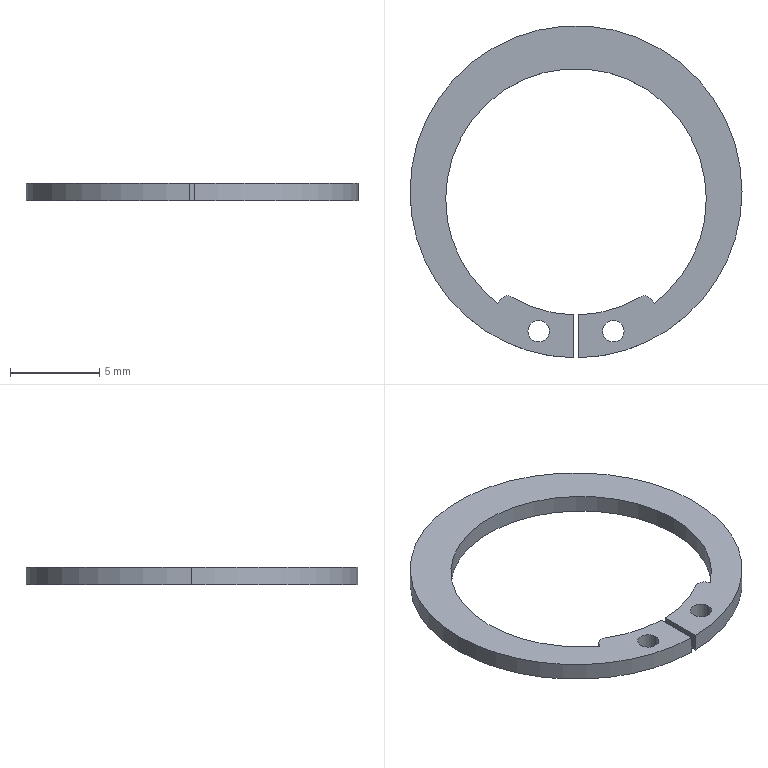Part | SolidWorks | features BaseBody 1 | 1 solid | 20 faces | box 18.6 x 18.599 x 1 mm | volume 108.117 mm3 | cylinder 14 | plane 6 | commonest cylinder face diameters 1.2 x4 14.6 x3 18.6 x3 1 x2 13.8 x2
STEP:
#1=CARTESIAN_POINT('',(7.3,-0.4,1.));
#2=VERTEX_POINT('',#1);
#3=CARTESIAN_POINT('',(4.373,-6.245,1.));
#4=VERTEX_POINT('',#3);
#5=CARTESIAN_POINT('',(0.,-0.4,1.));
#6=DIRECTION('',(0.,0.,-1.));
#7=DIRECTION('',(-1.,0.,0.));
#8=AXIS2_PLACEMENT_3D('',#5,#6,#7);
#9=CIRCLE('',#8,7.3);
#10=EDGE_CURVE('',#2,#4,#9,.T.);
#11=ORIENTED_EDGE('',*,*,#10,.F.);
#12=CARTESIAN_POINT('',(7.3,-0.4,0.));
#13=VERTEX_POINT('',#12);
#14=CARTESIAN_POINT('',(7.3,-0.4,1.));
#15=DIRECTION('',(0.,0.,-1.));
#16=VECTOR('',#15,1000.);
#17=LINE('',#14,#16);
#18=EDGE_CURVE('',#2,#13,#17,.T.);
#19=ORIENTED_EDGE('',*,*,#18,.T.);
#20=CARTESIAN_POINT('',(4.373,-6.245,0.));
#21=VERTEX_POINT('',#20);
#22=CARTESIAN_POINT('',(0.,-0.4,0.));
#23=DIRECTION('',(0.,0.,1.));
#24=DIRECTION('',(-1.,0.,0.));
#25=AXIS2_PLACEMENT_3D('',#22,#23,#24);
#26=CIRCLE('',#25,7.3);
#27=EDGE_CURVE('',#21,#13,#26,.T.);
#28=ORIENTED_EDGE('',*,*,#27,.F.);
#29=CARTESIAN_POINT('',(4.373,-6.245,1.));
#30=DIRECTION('',(0.,0.,1.));
#31=VECTOR('',#30,1000.);
#32=LINE('',#29,#31);
#33=EDGE_CURVE('',#21,#4,#32,.T.);
#34=ORIENTED_EDGE('',*,*,#33,.T.);
#35=EDGE_LOOP('',(#11,#19,#28,#34));
#36=FACE_OUTER_BOUND('',#35,.T.);
#37=CARTESIAN_POINT('',(0.,-0.4,1.));
#38=DIRECTION('',(0.,0.,-1.));
#39=DIRECTION('',(-1.,0.,0.));
#40=AXIS2_PLACEMENT_3D('',#37,#38,#39);
#41=CYLINDRICAL_SURFACE('',#40,7.3);
#42=ADVANCED_FACE('',(#36),#41,.F.);
#43=ORIENTED_EDGE('',*,*,#18,.F.);
#44=CARTESIAN_POINT('',(-7.3,-0.4,1.));
#45=VERTEX_POINT('',#44);
#46=CARTESIAN_POINT('',(0.,-0.4,1.));
#47=DIRECTION('',(0.,0.,-1.));
#48=DIRECTION('',(-1.,0.,0.));
#49=AXIS2_PLACEMENT_3D('',#46,#47,#48);
#50=CIRCLE('',#49,7.3);
#51=EDGE_CURVE('',#45,#2,#50,.T.);
#52=ORIENTED_EDGE('',*,*,#51,.F.);
#53=CARTESIAN_POINT('',(-7.3,-0.4,0.));
#54=VERTEX_POINT('',#53);
#55=CARTESIAN_POINT('',(-7.3,-0.4,1.));
#56=DIRECTION('',(0.,0.,-1.));
#57=VECTOR('',#56,1000.);
#58=LINE('',#55,#57);
#59=EDGE_CURVE('',#45,#54,#58,.T.);
#60=ORIENTED_EDGE('',*,*,#59,.T.);
#61=CARTESIAN_POINT('',(0.,-0.4,0.));
#62=DIRECTION('',(0.,0.,1.));
#63=DIRECTION('',(-1.,0.,0.));
#64=AXIS2_PLACEMENT_3D('',#61,#62,#63);
#65=CIRCLE('',#64,7.3);
#66=EDGE_CURVE('',#13,#54,#65,.T.);
#67=ORIENTED_EDGE('',*,*,#66,.F.);
#68=EDGE_LOOP('',(#43,#52,#60,#67));
#69=FACE_OUTER_BOUND('',#68,.T.);
#70=CARTESIAN_POINT('',(0.,-0.4,1.));
#71=DIRECTION('',(0.,0.,-1.));
#72=DIRECTION('',(-1.,0.,0.));
#73=AXIS2_PLACEMENT_3D('',#70,#71,#72);
#74=CYLINDRICAL_SURFACE('',#73,7.3);
#75=ADVANCED_FACE('',(#69),#74,.F.);
#76=CARTESIAN_POINT('',(9.3,0.,1.));
#77=VERTEX_POINT('',#76);
#78=CARTESIAN_POINT('',(-9.3,0.,1.));
#79=VERTEX_POINT('',#78);
#80=CARTESIAN_POINT('',(0.,0.,1.));
#81=DIRECTION('',(0.,0.,1.));
#82=DIRECTION('',(-1.,0.,0.));
#83=AXIS2_PLACEMENT_3D('',#80,#81,#82);
#84=CIRCLE('',#83,9.3);
#85=EDGE_CURVE('',#77,#79,#84,.T.);
#86=ORIENTED_EDGE('',*,*,#85,.F.);
#87=CARTESIAN_POINT('',(9.3,0.,0.));
#88=VERTEX_POINT('',#87);
#89=CARTESIAN_POINT('',(9.3,0.,1.));
#90=DIRECTION('',(0.,0.,-1.));
#91=VECTOR('',#90,1000.);
#92=LINE('',#89,#91);
#93=EDGE_CURVE('',#77,#88,#92,.T.);
#94=ORIENTED_EDGE('',*,*,#93,.T.);
#95=CARTESIAN_POINT('',(-9.3,0.,0.));
#96=VERTEX_POINT('',#95);
#97=CARTESIAN_POINT('',(0.,0.,0.));
#98=DIRECTION('',(0.,0.,1.));
#99=DIRECTION('',(-1.,0.,0.));
#100=AXIS2_PLACEMENT_3D('',#97,#98,#99);
#101=CIRCLE('',#100,9.3);
#102=EDGE_CURVE('',#88,#96,#101,.T.);
#103=ORIENTED_EDGE('',*,*,#102,.T.);
#104=CARTESIAN_POINT('',(-9.3,0.,1.));
#105=DIRECTION('',(0.,0.,-1.));
#106=VECTOR('',#105,1000.);
#107=LINE('',#104,#106);
#108=EDGE_CURVE('',#79,#96,#107,.T.);
#109=ORIENTED_EDGE('',*,*,#108,.F.);
#110=EDGE_LOOP('',(#86,#94,#103,#109));
#111=FACE_OUTER_BOUND('',#110,.T.);
#112=CARTESIAN_POINT('',(0.,0.,1.));
#113=DIRECTION('',(0.,0.,-1.));
#114=DIRECTION('',(-1.,0.,0.));
#115=AXIS2_PLACEMENT_3D('',#112,#113,#114);
#116=CYLINDRICAL_SURFACE('',#115,9.3);
#117=ADVANCED_FACE('',(#111),#116,.T.);
#118=CARTESIAN_POINT('',(-0.15,-9.299,1.));
#119=VERTEX_POINT('',#118);
#120=CARTESIAN_POINT('',(0.,0.,1.));
#121=DIRECTION('',(0.,0.,1.));
#122=DIRECTION('',(-1.,0.,0.));
#123=AXIS2_PLACEMENT_3D('',#120,#121,#122);
#124=CIRCLE('',#123,9.3);
#125=EDGE_CURVE('',#79,#119,#124,.T.);
#126=ORIENTED_EDGE('',*,*,#125,.F.);
#127=ORIENTED_EDGE('',*,*,#108,.T.);
#128=CARTESIAN_POINT('',(-0.15,-9.299,0.));
#129=VERTEX_POINT('',#128);
#130=CARTESIAN_POINT('',(0.,0.,0.));
#131=DIRECTION('',(0.,0.,1.));
#132=DIRECTION('',(-1.,0.,0.));
#133=AXIS2_PLACEMENT_3D('',#130,#131,#132);
#134=CIRCLE('',#133,9.3);
#135=EDGE_CURVE('',#96,#129,#134,.T.);
#136=ORIENTED_EDGE('',*,*,#135,.T.);
#137=CARTESIAN_POINT('',(-0.15,-9.299,1.));
#138=DIRECTION('',(0.,0.,1.));
#139=VECTOR('',#138,1000.);
#140=LINE('',#137,#139);
#141=EDGE_CURVE('',#129,#119,#140,.T.);
#142=ORIENTED_EDGE('',*,*,#141,.T.);
#143=EDGE_LOOP('',(#126,#127,#136,#142));
#144=FACE_OUTER_BOUND('',#143,.T.);
#145=CARTESIAN_POINT('',(0.,0.,1.));
#146=DIRECTION('',(0.,0.,-1.));
#147=DIRECTION('',(-1.,0.,0.));
#148=AXIS2_PLACEMENT_3D('',#145,#146,#147);
#149=CYLINDRICAL_SURFACE('',#148,9.3);
#150=ADVANCED_FACE('',(#144),#149,.T.);
#151=CARTESIAN_POINT('',(2.693,-7.811,1.));
#152=VERTEX_POINT('',#151);
#153=CARTESIAN_POINT('',(1.493,-7.811,1.));
#154=VERTEX_POINT('',#153);
#155=CARTESIAN_POINT('',(2.093,-7.811,1.));
#156=DIRECTION('',(0.,0.,-1.));
#157=DIRECTION('',(-1.,0.,0.));
#158=AXIS2_PLACEMENT_3D('',#155,#156,#157);
#159=CIRCLE('',#158,0.6);
#160=EDGE_CURVE('',#152,#154,#159,.T.);
#161=ORIENTED_EDGE('',*,*,#160,.F.);
#162=CARTESIAN_POINT('',(2.693,-7.811,0.));
#163=VERTEX_POINT('',#162);
#164=CARTESIAN_POINT('',(2.693,-7.811,1.));
#165=DIRECTION('',(0.,0.,-1.));
#166=VECTOR('',#165,1000.);
#167=LINE('',#164,#166);
#168=EDGE_CURVE('',#152,#163,#167,.T.);
#169=ORIENTED_EDGE('',*,*,#168,.T.);
#170=CARTESIAN_POINT('',(1.493,-7.811,0.));
#171=VERTEX_POINT('',#170);
#172=CARTESIAN_POINT('',(2.093,-7.811,0.));
#173=DIRECTION('',(0.,0.,1.));
#174=DIRECTION('',(-1.,0.,0.));
#175=AXIS2_PLACEMENT_3D('',#172,#173,#174);
#176=CIRCLE('',#175,0.6);
#177=EDGE_CURVE('',#171,#163,#176,.T.);
#178=ORIENTED_EDGE('',*,*,#177,.F.);
#179=CARTESIAN_POINT('',(1.493,-7.811,1.));
#180=DIRECTION('',(0.,0.,-1.));
#181=VECTOR('',#180,1000.);
#182=LINE('',#179,#181);
#183=EDGE_CURVE('',#154,#171,#182,.T.);
#184=ORIENTED_EDGE('',*,*,#183,.F.);
#185=EDGE_LOOP('',(#161,#169,#178,#184));
#186=FACE_OUTER_BOUND('',#185,.T.);
#187=CARTESIAN_POINT('',(2.093,-7.811,1.));
#188=DIRECTION('',(0.,0.,-1.));
#189=DIRECTION('',(-1.,0.,0.));
#190=AXIS2_PLACEMENT_3D('',#187,#188,#189);
#191=CYLINDRICAL_SURFACE('',#190,0.6);
#192=ADVANCED_FACE('',(#186),#191,.F.);
#193=CARTESIAN_POINT('',(-1.493,-7.811,1.));
#194=VERTEX_POINT('',#193);
#195=CARTESIAN_POINT('',(-2.693,-7.811,1.));
#196=VERTEX_POINT('',#195);
#197=CARTESIAN_POINT('',(-2.093,-7.811,1.));
#198=DIRECTION('',(0.,0.,-1.));
#199=DIRECTION('',(-1.,0.,0.));
#200=AXIS2_PLACEMENT_3D('',#197,#198,#199);
#201=CIRCLE('',#200,0.6);
#202=EDGE_CURVE('',#194,#196,#201,.T.);
#203=ORIENTED_EDGE('',*,*,#202,.F.);
#204=CARTESIAN_POINT('',(-1.493,-7.811,0.));
#205=VERTEX_POINT('',#204);
#206=CARTESIAN_POINT('',(-1.493,-7.811,1.));
#207=DIRECTION('',(0.,0.,-1.));
#208=VECTOR('',#207,1000.);
#209=LINE('',#206,#208);
#210=EDGE_CURVE('',#194,#205,#209,.T.);
#211=ORIENTED_EDGE('',*,*,#210,.T.);
#212=CARTESIAN_POINT('',(-2.693,-7.811,0.));
#213=VERTEX_POINT('',#212);
#214=CARTESIAN_POINT('',(-2.093,-7.811,0.));
#215=DIRECTION('',(0.,0.,1.));
#216=DIRECTION('',(-1.,0.,0.));
#217=AXIS2_PLACEMENT_3D('',#214,#215,#216);
#218=CIRCLE('',#217,0.6);
#219=EDGE_CURVE('',#213,#205,#218,.T.);
#220=ORIENTED_EDGE('',*,*,#219,.F.);
#221=CARTESIAN_POINT('',(-2.693,-7.811,1.));
#222=DIRECTION('',(0.,0.,-1.));
#223=VECTOR('',#222,1000.);
#224=LINE('',#221,#223);
#225=EDGE_CURVE('',#196,#213,#224,.T.);
#226=ORIENTED_EDGE('',*,*,#225,.F.);
#227=EDGE_LOOP('',(#203,#211,#220,#226));
#228=FACE_OUTER_BOUND('',#227,.T.);
#229=CARTESIAN_POINT('',(-2.093,-7.811,1.));
#230=DIRECTION('',(0.,0.,-1.));
#231=DIRECTION('',(-1.,0.,0.));
#232=AXIS2_PLACEMENT_3D('',#229,#230,#231);
#233=CYLINDRICAL_SURFACE('',#232,0.6);
#234=ADVANCED_FACE('',(#228),#233,.F.);
#235=ORIENTED_EDGE('',*,*,#219,.T.);
#236=CARTESIAN_POINT('',(-2.093,-7.811,0.));
#237=DIRECTION('',(0.,0.,1.));
#238=DIRECTION('',(-1.,0.,0.));
#239=AXIS2_PLACEMENT_3D('',#236,#237,#238);
#240=CIRCLE('',#239,0.6);
#241=EDGE_CURVE('',#205,#213,#240,.T.);
#242=ORIENTED_EDGE('',*,*,#241,.T.);
#243=EDGE_LOOP('',(#235,#242));
#244=FACE_BOUND('',#243,.T.);
#245=ORIENTED_EDGE('',*,*,#177,.T.);
#246=CARTESIAN_POINT('',(2.093,-7.811,0.));
#247=DIRECTION('',(0.,0.,1.));
#248=DIRECTION('',(-1.,0.,0.));
#249=AXIS2_PLACEMENT_3D('',#246,#247,#248);
#250=CIRCLE('',#249,0.6);
#251=EDGE_CURVE('',#163,#171,#250,.T.);
#252=ORIENTED_EDGE('',*,*,#251,.T.);
#253=EDGE_LOOP('',(#245,#252));
#254=FACE_BOUND('',#253,.T.);
#255=CARTESIAN_POINT('',(0.15,-6.898,0.));
#256=VERTEX_POINT('',#255);
#257=CARTESIAN_POINT('',(3.567,-5.907,0.));
#258=VERTEX_POINT('',#257);
#259=CARTESIAN_POINT('',(0.,0.,0.));
#260=DIRECTION('',(0.,0.,1.));
#261=DIRECTION('',(-1.,0.,0.));
#262=AXIS2_PLACEMENT_3D('',#259,#260,#261);
#263=CIRCLE('',#262,6.9);
#264=EDGE_CURVE('',#256,#258,#263,.T.);
#265=ORIENTED_EDGE('',*,*,#264,.T.);
#266=CARTESIAN_POINT('',(4.235,-6.048,0.));
#267=VERTEX_POINT('',#266);
#268=CARTESIAN_POINT('',(3.825,-6.335,0.));
#269=DIRECTION('',(0.,0.,1.));
#270=DIRECTION('',(-1.,0.,0.));
#271=AXIS2_PLACEMENT_3D('',#268,#269,#270);
#272=CIRCLE('',#271,0.5);
#273=EDGE_CURVE('',#267,#258,#272,.T.);
#274=ORIENTED_EDGE('',*,*,#273,.F.);
#275=CARTESIAN_POINT('',(4.373,-6.245,0.));
#276=DIRECTION('',(0.5736,-0.8192,0.));
#277=VECTOR('',#276,1000.);
#278=LINE('',#275,#277);
#279=EDGE_CURVE('',#267,#21,#278,.T.);
#280=ORIENTED_EDGE('',*,*,#279,.T.);
#281=ORIENTED_EDGE('',*,*,#27,.T.);
#282=ORIENTED_EDGE('',*,*,#66,.T.);
#283=CARTESIAN_POINT('',(-4.373,-6.245,0.));
#284=VERTEX_POINT('',#283);
#285=CARTESIAN_POINT('',(0.,-0.4,0.));
#286=DIRECTION('',(0.,0.,1.));
#287=DIRECTION('',(-1.,0.,0.));
#288=AXIS2_PLACEMENT_3D('',#285,#286,#287);
#289=CIRCLE('',#288,7.3);
#290=EDGE_CURVE('',#54,#284,#289,.T.);
#291=ORIENTED_EDGE('',*,*,#290,.T.);
#292=CARTESIAN_POINT('',(-4.235,-6.048,0.));
#293=VERTEX_POINT('',#292);
#294=CARTESIAN_POINT('',(-4.235,-6.048,0.));
#295=DIRECTION('',(0.5736,0.8192,0.));
#296=VECTOR('',#295,1000.);
#297=LINE('',#294,#296);
#298=EDGE_CURVE('',#284,#293,#297,.T.);
#299=ORIENTED_EDGE('',*,*,#298,.T.);
#300=CARTESIAN_POINT('',(-3.567,-5.907,0.));
#301=VERTEX_POINT('',#300);
#302=CARTESIAN_POINT('',(-3.825,-6.335,0.));
#303=DIRECTION('',(0.,0.,1.));
#304=DIRECTION('',(-1.,0.,0.));
#305=AXIS2_PLACEMENT_3D('',#302,#303,#304);
#306=CIRCLE('',#305,0.5);
#307=EDGE_CURVE('',#301,#293,#306,.T.);
#308=ORIENTED_EDGE('',*,*,#307,.F.);
#309=CARTESIAN_POINT('',(-0.15,-6.898,0.));
#310=VERTEX_POINT('',#309);
#311=CARTESIAN_POINT('',(0.,0.,0.));
#312=DIRECTION('',(0.,0.,1.));
#313=DIRECTION('',(-1.,0.,0.));
#314=AXIS2_PLACEMENT_3D('',#311,#312,#313);
#315=CIRCLE('',#314,6.9);
#316=EDGE_CURVE('',#301,#310,#315,.T.);
#317=ORIENTED_EDGE('',*,*,#316,.T.);
#318=CARTESIAN_POINT('',(-0.15,-9.299,0.));
#319=DIRECTION('',(0.,-1.,0.));
#320=VECTOR('',#319,1000.);
#321=LINE('',#318,#320);
#322=EDGE_CURVE('',#310,#129,#321,.T.);
#323=ORIENTED_EDGE('',*,*,#322,.T.);
#324=ORIENTED_EDGE('',*,*,#135,.F.);
#325=ORIENTED_EDGE('',*,*,#102,.F.);
#326=CARTESIAN_POINT('',(0.15,-9.299,0.));
#327=VERTEX_POINT('',#326);
#328=CARTESIAN_POINT('',(0.,0.,0.));
#329=DIRECTION('',(0.,0.,1.));
#330=DIRECTION('',(-1.,0.,0.));
#331=AXIS2_PLACEMENT_3D('',#328,#329,#330);
#332=CIRCLE('',#331,9.3);
#333=EDGE_CURVE('',#327,#88,#332,.T.);
#334=ORIENTED_EDGE('',*,*,#333,.F.);
#335=CARTESIAN_POINT('',(0.15,-6.898,0.));
#336=DIRECTION('',(0.,1.,0.));
#337=VECTOR('',#336,1000.);
#338=LINE('',#335,#337);
#339=EDGE_CURVE('',#327,#256,#338,.T.);
#340=ORIENTED_EDGE('',*,*,#339,.T.);
#341=EDGE_LOOP('',(#265,#274,#280,#281,#282,#291,#299,#308,#317,#323,#324,#325,#334,#340));
#342=FACE_OUTER_BOUND('',#341,.T.);
#343=CARTESIAN_POINT('',(0.,0.,0.));
#344=DIRECTION('',(0.,0.,1.));
#345=DIRECTION('',(1.,0.,0.));
#346=AXIS2_PLACEMENT_3D('',#343,#344,#345);
#347=PLANE('',#346);
#348=ADVANCED_FACE('',(#244,#254,#342),#347,.F.);
#349=CARTESIAN_POINT('',(0.15,-9.299,1.));
#350=VERTEX_POINT('',#349);
#351=CARTESIAN_POINT('',(0.15,-9.299,1.));
#352=DIRECTION('',(0.,0.,-1.));
#353=VECTOR('',#352,1000.);
#354=LINE('',#351,#353);
#355=EDGE_CURVE('',#350,#327,#354,.T.);
#356=ORIENTED_EDGE('',*,*,#355,.F.);
#357=CARTESIAN_POINT('',(0.15,-6.898,1.));
#358=VERTEX_POINT('',#357);
#359=CARTESIAN_POINT('',(0.15,0.,1.));
#360=DIRECTION('',(0.,-1.,0.));
#361=VECTOR('',#360,1000.);
#362=LINE('',#359,#361);
#363=EDGE_CURVE('',#358,#350,#362,.T.);
#364=ORIENTED_EDGE('',*,*,#363,.F.);
#365=CARTESIAN_POINT('',(0.15,-6.898,1.));
#366=DIRECTION('',(0.,0.,-1.));
#367=VECTOR('',#366,1000.);
#368=LINE('',#365,#367);
#369=EDGE_CURVE('',#358,#256,#368,.T.);
#370=ORIENTED_EDGE('',*,*,#369,.T.);
#371=ORIENTED_EDGE('',*,*,#339,.F.);
#372=EDGE_LOOP('',(#356,#364,#370,#371));
#373=FACE_OUTER_BOUND('',#372,.T.);
#374=CARTESIAN_POINT('',(0.15,-6.898,1.));
#375=DIRECTION('',(1.,0.,0.));
#376=DIRECTION('',(0.,1.,0.));
#377=AXIS2_PLACEMENT_3D('',#374,#375,#376);
#378=PLANE('',#377);
#379=ADVANCED_FACE('',(#373),#378,.F.);
#380=CARTESIAN_POINT('',(-0.15,-6.898,1.));
#381=VERTEX_POINT('',#380);
#382=CARTESIAN_POINT('',(-0.15,-6.898,1.));
#383=DIRECTION('',(0.,0.,1.));
#384=VECTOR('',#383,1000.);
#385=LINE('',#382,#384);
#386=EDGE_CURVE('',#310,#381,#385,.T.);
#387=ORIENTED_EDGE('',*,*,#386,.T.);
#388=CARTESIAN_POINT('',(-0.15,0.,1.));
#389=DIRECTION('',(0.,1.,0.));
#390=VECTOR('',#389,1000.);
#391=LINE('',#388,#390);
#392=EDGE_CURVE('',#119,#381,#391,.T.);
#393=ORIENTED_EDGE('',*,*,#392,.F.);
#394=ORIENTED_EDGE('',*,*,#141,.F.);
#395=ORIENTED_EDGE('',*,*,#322,.F.);
#396=EDGE_LOOP('',(#387,#393,#394,#395));
#397=FACE_OUTER_BOUND('',#396,.T.);
#398=CARTESIAN_POINT('',(-0.15,-9.299,1.));
#399=DIRECTION('',(-1.,0.,0.));
#400=DIRECTION('',(0.,0.,1.));
#401=AXIS2_PLACEMENT_3D('',#398,#399,#400);
#402=PLANE('',#401);
#403=ADVANCED_FACE('',(#397),#402,.F.);
#404=CARTESIAN_POINT('',(-3.567,-5.907,1.));
#405=VERTEX_POINT('',#404);
#406=CARTESIAN_POINT('',(-3.567,-5.907,1.));
#407=DIRECTION('',(0.,0.,-1.));
#408=VECTOR('',#407,1000.);
#409=LINE('',#406,#408);
#410=EDGE_CURVE('',#405,#301,#409,.T.);
#411=ORIENTED_EDGE('',*,*,#410,.F.);
#412=CARTESIAN_POINT('',(0.,0.,1.));
#413=DIRECTION('',(0.,0.,-1.));
#414=DIRECTION('',(-1.,0.,0.));
#415=AXIS2_PLACEMENT_3D('',#412,#413,#414);
#416=CIRCLE('',#415,6.9);
#417=EDGE_CURVE('',#381,#405,#416,.T.);
#418=ORIENTED_EDGE('',*,*,#417,.F.);
#419=ORIENTED_EDGE('',*,*,#386,.F.);
#420=ORIENTED_EDGE('',*,*,#316,.F.);
#421=EDGE_LOOP('',(#411,#418,#419,#420));
#422=FACE_OUTER_BOUND('',#421,.T.);
#423=CARTESIAN_POINT('',(0.,0.,1.));
#424=DIRECTION('',(0.,0.,-1.));
#425=DIRECTION('',(-1.,0.,0.));
#426=AXIS2_PLACEMENT_3D('',#423,#424,#425);
#427=CYLINDRICAL_SURFACE('',#426,6.9);
#428=ADVANCED_FACE('',(#422),#427,.F.);
#429=CARTESIAN_POINT('',(-4.235,-6.048,1.));
#430=VERTEX_POINT('',#429);
#431=CARTESIAN_POINT('',(-3.825,-6.335,1.));
#432=DIRECTION('',(0.,0.,1.));
#433=DIRECTION('',(-1.,0.,0.));
#434=AXIS2_PLACEMENT_3D('',#431,#432,#433);
#435=CIRCLE('',#434,0.5);
#436=EDGE_CURVE('',#405,#430,#435,.T.);
#437=ORIENTED_EDGE('',*,*,#436,.F.);
#438=ORIENTED_EDGE('',*,*,#410,.T.);
#439=ORIENTED_EDGE('',*,*,#307,.T.);
#440=CARTESIAN_POINT('',(-4.235,-6.048,1.));
#441=DIRECTION('',(0.,0.,1.));
#442=VECTOR('',#441,1000.);
#443=LINE('',#440,#442);
#444=EDGE_CURVE('',#293,#430,#443,.T.);
#445=ORIENTED_EDGE('',*,*,#444,.T.);
#446=EDGE_LOOP('',(#437,#438,#439,#445));
#447=FACE_OUTER_BOUND('',#446,.T.);
#448=CARTESIAN_POINT('',(-3.825,-6.335,1.));
#449=DIRECTION('',(0.,0.,-1.));
#450=DIRECTION('',(-1.,0.,0.));
#451=AXIS2_PLACEMENT_3D('',#448,#449,#450);
#452=CYLINDRICAL_SURFACE('',#451,0.5);
#453=ADVANCED_FACE('',(#447),#452,.T.);
#454=CARTESIAN_POINT('',(-4.373,-6.245,1.));
#455=VERTEX_POINT('',#454);
#456=CARTESIAN_POINT('',(-4.373,-6.245,1.));
#457=DIRECTION('',(0.,0.,1.));
#458=VECTOR('',#457,1000.);
#459=LINE('',#456,#458);
#460=EDGE_CURVE('',#284,#455,#459,.T.);
#461=ORIENTED_EDGE('',*,*,#460,.T.);
#462=CARTESIAN_POINT('',(-4.235,-6.048,1.));
#463=DIRECTION('',(-0.5736,-0.8192,0.));
#464=VECTOR('',#463,1000.);
#465=LINE('',#462,#464);
#466=EDGE_CURVE('',#430,#455,#465,.T.);
#467=ORIENTED_EDGE('',*,*,#466,.F.);
#468=ORIENTED_EDGE('',*,*,#444,.F.);
#469=ORIENTED_EDGE('',*,*,#298,.F.);
#470=EDGE_LOOP('',(#461,#467,#468,#469));
#471=FACE_OUTER_BOUND('',#470,.T.);
#472=CARTESIAN_POINT('',(-4.235,-6.048,1.));
#473=DIRECTION('',(0.8192,-0.5736,0.));
#474=DIRECTION('',(0.,0.,-1.));
#475=AXIS2_PLACEMENT_3D('',#472,#473,#474);
#476=PLANE('',#475);
#477=ADVANCED_FACE('',(#471),#476,.F.);
#478=CARTESIAN_POINT('',(4.235,-6.048,1.));
#479=VERTEX_POINT('',#478);
#480=CARTESIAN_POINT('',(4.235,-6.048,1.));
#481=DIRECTION('',(0.,0.,-1.));
#482=VECTOR('',#481,1000.);
#483=LINE('',#480,#482);
#484=EDGE_CURVE('',#479,#267,#483,.T.);
#485=ORIENTED_EDGE('',*,*,#484,.F.);
#486=CARTESIAN_POINT('',(4.373,-6.245,1.));
#487=DIRECTION('',(-0.5736,0.8192,0.));
#488=VECTOR('',#487,1000.);
#489=LINE('',#486,#488);
#490=EDGE_CURVE('',#4,#479,#489,.T.);
#491=ORIENTED_EDGE('',*,*,#490,.F.);
#492=ORIENTED_EDGE('',*,*,#33,.F.);
#493=ORIENTED_EDGE('',*,*,#279,.F.);
#494=EDGE_LOOP('',(#485,#491,#492,#493));
#495=FACE_OUTER_BOUND('',#494,.T.);
#496=CARTESIAN_POINT('',(4.373,-6.245,1.));
#497=DIRECTION('',(-0.8192,-0.5736,0.));
#498=DIRECTION('',(-0.5736,0.8192,0.));
#499=AXIS2_PLACEMENT_3D('',#496,#497,#498);
#500=PLANE('',#499);
#501=ADVANCED_FACE('',(#495),#500,.F.);
#502=CARTESIAN_POINT('',(3.567,-5.907,1.));
#503=VERTEX_POINT('',#502);
#504=CARTESIAN_POINT('',(3.825,-6.335,1.));
#505=DIRECTION('',(0.,0.,1.));
#506=DIRECTION('',(-1.,0.,0.));
#507=AXIS2_PLACEMENT_3D('',#504,#505,#506);
#508=CIRCLE('',#507,0.5);
#509=EDGE_CURVE('',#479,#503,#508,.T.);
#510=ORIENTED_EDGE('',*,*,#509,.F.);
#511=ORIENTED_EDGE('',*,*,#484,.T.);
#512=ORIENTED_EDGE('',*,*,#273,.T.);
#513=CARTESIAN_POINT('',(3.567,-5.907,1.));
#514=DIRECTION('',(0.,0.,1.));
#515=VECTOR('',#514,1000.);
#516=LINE('',#513,#515);
#517=EDGE_CURVE('',#258,#503,#516,.T.);
#518=ORIENTED_EDGE('',*,*,#517,.T.);
#519=EDGE_LOOP('',(#510,#511,#512,#518));
#520=FACE_OUTER_BOUND('',#519,.T.);
#521=CARTESIAN_POINT('',(3.825,-6.335,1.));
#522=DIRECTION('',(0.,0.,-1.));
#523=DIRECTION('',(-1.,0.,0.));
#524=AXIS2_PLACEMENT_3D('',#521,#522,#523);
#525=CYLINDRICAL_SURFACE('',#524,0.5);
#526=ADVANCED_FACE('',(#520),#525,.T.);
#527=ORIENTED_EDGE('',*,*,#369,.F.);
#528=CARTESIAN_POINT('',(0.,0.,1.));
#529=DIRECTION('',(0.,0.,-1.));
#530=DIRECTION('',(-1.,0.,0.));
#531=AXIS2_PLACEMENT_3D('',#528,#529,#530);
#532=CIRCLE('',#531,6.9);
#533=EDGE_CURVE('',#503,#358,#532,.T.);
#534=ORIENTED_EDGE('',*,*,#533,.F.);
#535=ORIENTED_EDGE('',*,*,#517,.F.);
#536=ORIENTED_EDGE('',*,*,#264,.F.);
#537=EDGE_LOOP('',(#527,#534,#535,#536));
#538=FACE_OUTER_BOUND('',#537,.T.);
#539=CARTESIAN_POINT('',(0.,0.,1.));
#540=DIRECTION('',(0.,0.,-1.));
#541=DIRECTION('',(-1.,0.,0.));
#542=AXIS2_PLACEMENT_3D('',#539,#540,#541);
#543=CYLINDRICAL_SURFACE('',#542,6.9);
#544=ADVANCED_FACE('',(#538),#543,.F.);
#545=CARTESIAN_POINT('',(-2.093,-7.811,1.));
#546=DIRECTION('',(0.,0.,-1.));
#547=DIRECTION('',(-1.,0.,0.));
#548=AXIS2_PLACEMENT_3D('',#545,#546,#547);
#549=CIRCLE('',#548,0.6);
#550=EDGE_CURVE('',#196,#194,#549,.T.);
#551=ORIENTED_EDGE('',*,*,#550,.T.);
#552=ORIENTED_EDGE('',*,*,#202,.T.);
#553=EDGE_LOOP('',(#551,#552));
#554=FACE_BOUND('',#553,.T.);
#555=CARTESIAN_POINT('',(2.093,-7.811,1.));
#556=DIRECTION('',(0.,0.,-1.));
#557=DIRECTION('',(-1.,0.,0.));
#558=AXIS2_PLACEMENT_3D('',#555,#556,#557);
#559=CIRCLE('',#558,0.6);
#560=EDGE_CURVE('',#154,#152,#559,.T.);
#561=ORIENTED_EDGE('',*,*,#560,.T.);
#562=ORIENTED_EDGE('',*,*,#160,.T.);
#563=EDGE_LOOP('',(#561,#562));
#564=FACE_BOUND('',#563,.T.);
#565=ORIENTED_EDGE('',*,*,#509,.T.);
#566=ORIENTED_EDGE('',*,*,#533,.T.);
#567=ORIENTED_EDGE('',*,*,#363,.T.);
#568=CARTESIAN_POINT('',(0.,0.,1.));
#569=DIRECTION('',(0.,0.,1.));
#570=DIRECTION('',(-1.,0.,0.));
#571=AXIS2_PLACEMENT_3D('',#568,#569,#570);
#572=CIRCLE('',#571,9.3);
#573=EDGE_CURVE('',#350,#77,#572,.T.);
#574=ORIENTED_EDGE('',*,*,#573,.T.);
#575=ORIENTED_EDGE('',*,*,#85,.T.);
#576=ORIENTED_EDGE('',*,*,#125,.T.);
#577=ORIENTED_EDGE('',*,*,#392,.T.);
#578=ORIENTED_EDGE('',*,*,#417,.T.);
#579=ORIENTED_EDGE('',*,*,#436,.T.);
#580=ORIENTED_EDGE('',*,*,#466,.T.);
#581=CARTESIAN_POINT('',(0.,-0.4,1.));
#582=DIRECTION('',(0.,0.,-1.));
#583=DIRECTION('',(-1.,0.,0.));
#584=AXIS2_PLACEMENT_3D('',#581,#582,#583);
#585=CIRCLE('',#584,7.3);
#586=EDGE_CURVE('',#455,#45,#585,.T.);
#587=ORIENTED_EDGE('',*,*,#586,.T.);
#588=ORIENTED_EDGE('',*,*,#51,.T.);
#589=ORIENTED_EDGE('',*,*,#10,.T.);
#590=ORIENTED_EDGE('',*,*,#490,.T.);
#591=EDGE_LOOP('',(#565,#566,#567,#574,#575,#576,#577,#578,#579,#580,#587,#588,#589,#590));
#592=FACE_OUTER_BOUND('',#591,.T.);
#593=CARTESIAN_POINT('',(0.,0.,1.));
#594=DIRECTION('',(0.,0.,1.));
#595=DIRECTION('',(1.,0.,0.));
#596=AXIS2_PLACEMENT_3D('',#593,#594,#595);
#597=PLANE('',#596);
#598=ADVANCED_FACE('',(#554,#564,#592),#597,.T.);
#599=ORIENTED_EDGE('',*,*,#210,.F.);
#600=ORIENTED_EDGE('',*,*,#550,.F.);
#601=ORIENTED_EDGE('',*,*,#225,.T.);
#602=ORIENTED_EDGE('',*,*,#241,.F.);
#603=EDGE_LOOP('',(#599,#600,#601,#602));
#604=FACE_OUTER_BOUND('',#603,.T.);
#605=CARTESIAN_POINT('',(-2.093,-7.811,1.));
#606=DIRECTION('',(0.,0.,-1.));
#607=DIRECTION('',(-1.,0.,0.));
#608=AXIS2_PLACEMENT_3D('',#605,#606,#607);
#609=CYLINDRICAL_SURFACE('',#608,0.6);
#610=ADVANCED_FACE('',(#604),#609,.F.);
#611=ORIENTED_EDGE('',*,*,#168,.F.);
#612=ORIENTED_EDGE('',*,*,#560,.F.);
#613=ORIENTED_EDGE('',*,*,#183,.T.);
#614=ORIENTED_EDGE('',*,*,#251,.F.);
#615=EDGE_LOOP('',(#611,#612,#613,#614));
#616=FACE_OUTER_BOUND('',#615,.T.);
#617=CARTESIAN_POINT('',(2.093,-7.811,1.));
#618=DIRECTION('',(0.,0.,-1.));
#619=DIRECTION('',(-1.,0.,0.));
#620=AXIS2_PLACEMENT_3D('',#617,#618,#619);
#621=CYLINDRICAL_SURFACE('',#620,0.6);
#622=ADVANCED_FACE('',(#616),#621,.F.);
#623=ORIENTED_EDGE('',*,*,#93,.F.);
#624=ORIENTED_EDGE('',*,*,#573,.F.);
#625=ORIENTED_EDGE('',*,*,#355,.T.);
#626=ORIENTED_EDGE('',*,*,#333,.T.);
#627=EDGE_LOOP('',(#623,#624,#625,#626));
#628=FACE_OUTER_BOUND('',#627,.T.);
#629=CARTESIAN_POINT('',(0.,0.,1.));
#630=DIRECTION('',(0.,0.,-1.));
#631=DIRECTION('',(-1.,0.,0.));
#632=AXIS2_PLACEMENT_3D('',#629,#630,#631);
#633=CYLINDRICAL_SURFACE('',#632,9.3);
#634=ADVANCED_FACE('',(#628),#633,.T.);
#635=ORIENTED_EDGE('',*,*,#59,.F.);
#636=ORIENTED_EDGE('',*,*,#586,.F.);
#637=ORIENTED_EDGE('',*,*,#460,.F.);
#638=ORIENTED_EDGE('',*,*,#290,.F.);
#639=EDGE_LOOP('',(#635,#636,#637,#638));
#640=FACE_OUTER_BOUND('',#639,.T.);
#641=CARTESIAN_POINT('',(0.,-0.4,1.));
#642=DIRECTION('',(0.,0.,-1.));
#643=DIRECTION('',(-1.,0.,0.));
#644=AXIS2_PLACEMENT_3D('',#641,#642,#643);
#645=CYLINDRICAL_SURFACE('',#644,7.3);
#646=ADVANCED_FACE('',(#640),#645,.F.);
#647=CLOSED_SHELL('',(#42,#75,#117,#150,#192,#234,#348,#379,#403,#428,#453,#477,#501,#526,#544,#598,#610,#622,#634,#646));
#648=MANIFOLD_SOLID_BREP('',#647);
#649=CARTESIAN_POINT('',(0.,0.,0.));
#650=DIRECTION('',(0.,0.,1.));
#651=DIRECTION('',(1.,0.,0.));
#652=AXIS2_PLACEMENT_3D('',#649,#650,#651);
#653=(LENGTH_UNIT()NAMED_UNIT(*)SI_UNIT(.MILLI.,.METRE.));
#654=UNCERTAINTY_MEASURE_WITH_UNIT(LENGTH_MEASURE(0.00001),#653,'','');
#655=(NAMED_UNIT(*)PLANE_ANGLE_UNIT()SI_UNIT($,.RADIAN.));
#656=(NAMED_UNIT(*)SI_UNIT($,.STERADIAN.)SOLID_ANGLE_UNIT());
#657=(GEOMETRIC_REPRESENTATION_CONTEXT(3)GLOBAL_UNCERTAINTY_ASSIGNED_CONTEXT((#654))GLOBAL_UNIT_ASSIGNED_CONTEXT((#653,#655,#656))REPRESENTATION_CONTEXT('',''));
#658=ADVANCED_BREP_SHAPE_REPRESENTATION('',(#648,#652),#657);